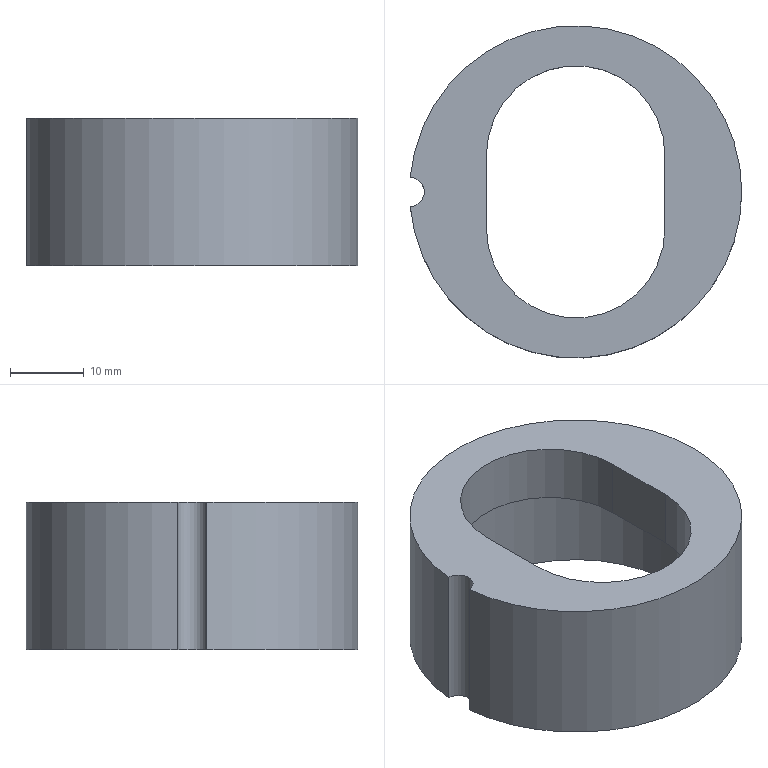Part | NX | features solid 2 | 1 solid | 10 faces | box 44.911 x 45 x 20 mm | volume 13855 mm3 | cylinder 5 | plane 5 | commonest cylinder face diameters 24.2 x2 4 x1 36 x1 45 x1
STEP:
#1=CARTESIAN_POINT('',(32.413,-54.637,-113.));
#2=VERTEX_POINT('',#1);
#3=CARTESIAN_POINT('',(32.413,-54.637,-93.));
#4=VERTEX_POINT('',#3);
#5=CARTESIAN_POINT('',(32.413,-54.637,-103.));
#6=DIRECTION('',(0.,0.,1.));
#7=VECTOR('',#6,1000.);
#8=LINE('',#5,#7);
#9=EDGE_CURVE('',#2,#4,#8,.T.);
#10=ORIENTED_EDGE('',*,*,#9,.F.);
#11=CARTESIAN_POINT('',(32.413,-50.641,-113.));
#12=VERTEX_POINT('',#11);
#13=CARTESIAN_POINT('',(54.824,-52.639,-113.));
#14=DIRECTION('',(0.,0.,1.));
#15=DIRECTION('',(-1.,0.,0.));
#16=AXIS2_PLACEMENT_3D('',#13,#14,#15);
#17=CIRCLE('',#16,22.5);
#18=EDGE_CURVE('',#2,#12,#17,.T.);
#19=ORIENTED_EDGE('',*,*,#18,.T.);
#20=CARTESIAN_POINT('',(32.413,-50.641,-93.));
#21=VERTEX_POINT('',#20);
#22=CARTESIAN_POINT('',(32.413,-50.641,-103.));
#23=DIRECTION('',(0.,0.,1.));
#24=VECTOR('',#23,1000.);
#25=LINE('',#22,#24);
#26=EDGE_CURVE('',#21,#12,#25,.F.);
#27=ORIENTED_EDGE('',*,*,#26,.F.);
#28=CARTESIAN_POINT('',(54.824,-52.639,-93.));
#29=DIRECTION('',(0.,0.,1.));
#30=DIRECTION('',(-1.,0.,0.));
#31=AXIS2_PLACEMENT_3D('',#28,#29,#30);
#32=CIRCLE('',#31,22.5);
#33=EDGE_CURVE('',#4,#21,#32,.T.);
#34=ORIENTED_EDGE('',*,*,#33,.F.);
#35=EDGE_LOOP('',(#10,#19,#27,#34));
#36=FACE_BOUND('',#35,.T.);
#37=CARTESIAN_POINT('',(54.824,-52.639,-113.));
#38=DIRECTION('',(0.,0.,1.));
#39=DIRECTION('',(-1.,0.,0.));
#40=AXIS2_PLACEMENT_3D('',#37,#38,#39);
#41=CYLINDRICAL_SURFACE('',#40,22.5);
#42=ADVANCED_FACE('',(#36),#41,.T.);
#43=CARTESIAN_POINT('',(36.824,-52.639,-113.));
#44=VERTEX_POINT('',#43);
#45=CARTESIAN_POINT('',(54.824,-52.639,-113.));
#46=DIRECTION('',(0.,0.,1.));
#47=DIRECTION('',(-1.,0.,0.));
#48=AXIS2_PLACEMENT_3D('',#45,#46,#47);
#49=CIRCLE('',#48,18.);
#50=EDGE_CURVE('',#44,#44,#49,.T.);
#51=ORIENTED_EDGE('',*,*,#50,.T.);
#52=EDGE_LOOP('',(#51));
#53=FACE_BOUND('',#52,.T.);
#54=ORIENTED_EDGE('',*,*,#18,.F.);
#55=CARTESIAN_POINT('',(32.324,-52.639,-113.));
#56=DIRECTION('',(0.,0.,1.));
#57=DIRECTION('',(-1.,0.,0.));
#58=AXIS2_PLACEMENT_3D('',#55,#56,#57);
#59=CIRCLE('',#58,2.);
#60=EDGE_CURVE('',#2,#12,#59,.T.);
#61=ORIENTED_EDGE('',*,*,#60,.T.);
#62=EDGE_LOOP('',(#54,#61));
#63=FACE_BOUND('',#62,.T.);
#64=CARTESIAN_POINT('',(54.824,-52.639,-113.));
#65=DIRECTION('',(0.,0.,1.));
#66=DIRECTION('',(-1.,0.,0.));
#67=AXIS2_PLACEMENT_3D('',#64,#65,#66);
#68=PLANE('',#67);
#69=ADVANCED_FACE('',(#53,#63),#68,.F.);
#70=CARTESIAN_POINT('',(66.924,-57.639,-93.));
#71=VERTEX_POINT('',#70);
#72=CARTESIAN_POINT('',(66.924,-47.639,-93.));
#73=VERTEX_POINT('',#72);
#74=CARTESIAN_POINT('',(66.924,-57.639,-93.));
#75=DIRECTION('',(0.,1.,0.));
#76=VECTOR('',#75,1000.);
#77=LINE('',#74,#76);
#78=EDGE_CURVE('',#71,#73,#77,.T.);
#79=ORIENTED_EDGE('',*,*,#78,.F.);
#80=CARTESIAN_POINT('',(42.724,-57.639,-93.));
#81=VERTEX_POINT('',#80);
#82=CARTESIAN_POINT('',(54.824,-57.639,-93.));
#83=DIRECTION('',(0.,0.,1.));
#84=DIRECTION('',(-1.,0.,0.));
#85=AXIS2_PLACEMENT_3D('',#82,#83,#84);
#86=CIRCLE('',#85,12.1);
#87=EDGE_CURVE('',#81,#71,#86,.T.);
#88=ORIENTED_EDGE('',*,*,#87,.F.);
#89=CARTESIAN_POINT('',(42.724,-47.639,-93.));
#90=VERTEX_POINT('',#89);
#91=CARTESIAN_POINT('',(42.724,-57.639,-93.));
#92=DIRECTION('',(0.,1.,0.));
#93=VECTOR('',#92,1000.);
#94=LINE('',#91,#93);
#95=EDGE_CURVE('',#81,#90,#94,.T.);
#96=ORIENTED_EDGE('',*,*,#95,.T.);
#97=CARTESIAN_POINT('',(54.824,-47.639,-93.));
#98=DIRECTION('',(0.,0.,1.));
#99=DIRECTION('',(-1.,0.,0.));
#100=AXIS2_PLACEMENT_3D('',#97,#98,#99);
#101=CIRCLE('',#100,12.1);
#102=EDGE_CURVE('',#73,#90,#101,.T.);
#103=ORIENTED_EDGE('',*,*,#102,.F.);
#104=EDGE_LOOP('',(#79,#88,#96,#103));
#105=FACE_BOUND('',#104,.T.);
#106=CARTESIAN_POINT('',(32.324,-52.639,-93.));
#107=DIRECTION('',(0.,0.,1.));
#108=DIRECTION('',(-1.,0.,0.));
#109=AXIS2_PLACEMENT_3D('',#106,#107,#108);
#110=CIRCLE('',#109,2.);
#111=EDGE_CURVE('',#4,#21,#110,.T.);
#112=ORIENTED_EDGE('',*,*,#111,.F.);
#113=ORIENTED_EDGE('',*,*,#33,.T.);
#114=EDGE_LOOP('',(#112,#113));
#115=FACE_BOUND('',#114,.T.);
#116=CARTESIAN_POINT('',(54.824,-52.639,-93.));
#117=DIRECTION('',(0.,0.,1.));
#118=DIRECTION('',(-1.,0.,0.));
#119=AXIS2_PLACEMENT_3D('',#116,#117,#118);
#120=PLANE('',#119);
#121=ADVANCED_FACE('',(#105,#115),#120,.T.);
#122=ORIENTED_EDGE('',*,*,#50,.F.);
#123=EDGE_LOOP('',(#122));
#124=FACE_BOUND('',#123,.T.);
#125=CARTESIAN_POINT('',(36.824,-52.639,-101.));
#126=VERTEX_POINT('',#125);
#127=CARTESIAN_POINT('',(54.824,-52.639,-101.));
#128=DIRECTION('',(0.,0.,1.));
#129=DIRECTION('',(-1.,0.,0.));
#130=AXIS2_PLACEMENT_3D('',#127,#128,#129);
#131=CIRCLE('',#130,18.);
#132=EDGE_CURVE('',#126,#126,#131,.T.);
#133=ORIENTED_EDGE('',*,*,#132,.T.);
#134=EDGE_LOOP('',(#133));
#135=FACE_BOUND('',#134,.T.);
#136=CARTESIAN_POINT('',(54.824,-52.639,-113.));
#137=DIRECTION('',(0.,0.,1.));
#138=DIRECTION('',(-1.,0.,0.));
#139=AXIS2_PLACEMENT_3D('',#136,#137,#138);
#140=CYLINDRICAL_SURFACE('',#139,18.);
#141=ADVANCED_FACE('',(#124,#135),#140,.F.);
#142=CARTESIAN_POINT('',(42.724,-57.639,-101.));
#143=VERTEX_POINT('',#142);
#144=CARTESIAN_POINT('',(66.924,-57.639,-101.));
#145=VERTEX_POINT('',#144);
#146=CARTESIAN_POINT('',(54.824,-57.639,-101.));
#147=DIRECTION('',(0.,0.,1.));
#148=DIRECTION('',(-1.,0.,0.));
#149=AXIS2_PLACEMENT_3D('',#146,#147,#148);
#150=CIRCLE('',#149,12.1);
#151=EDGE_CURVE('',#143,#145,#150,.T.);
#152=ORIENTED_EDGE('',*,*,#151,.T.);
#153=CARTESIAN_POINT('',(66.924,-47.639,-101.));
#154=VERTEX_POINT('',#153);
#155=CARTESIAN_POINT('',(66.924,-52.639,-101.));
#156=DIRECTION('',(0.,1.,0.));
#157=VECTOR('',#156,1000.);
#158=LINE('',#155,#157);
#159=EDGE_CURVE('',#145,#154,#158,.T.);
#160=ORIENTED_EDGE('',*,*,#159,.T.);
#161=CARTESIAN_POINT('',(42.724,-47.639,-101.));
#162=VERTEX_POINT('',#161);
#163=CARTESIAN_POINT('',(54.824,-47.639,-101.));
#164=DIRECTION('',(0.,0.,1.));
#165=DIRECTION('',(-1.,0.,0.));
#166=AXIS2_PLACEMENT_3D('',#163,#164,#165);
#167=CIRCLE('',#166,12.1);
#168=EDGE_CURVE('',#154,#162,#167,.T.);
#169=ORIENTED_EDGE('',*,*,#168,.T.);
#170=CARTESIAN_POINT('',(42.724,-52.639,-101.));
#171=DIRECTION('',(0.,1.,0.));
#172=VECTOR('',#171,1000.);
#173=LINE('',#170,#172);
#174=EDGE_CURVE('',#143,#162,#173,.T.);
#175=ORIENTED_EDGE('',*,*,#174,.F.);
#176=EDGE_LOOP('',(#152,#160,#169,#175));
#177=FACE_BOUND('',#176,.T.);
#178=ORIENTED_EDGE('',*,*,#132,.F.);
#179=EDGE_LOOP('',(#178));
#180=FACE_BOUND('',#179,.T.);
#181=CARTESIAN_POINT('',(54.824,-52.639,-101.));
#182=DIRECTION('',(0.,0.,1.));
#183=DIRECTION('',(-1.,0.,0.));
#184=AXIS2_PLACEMENT_3D('',#181,#182,#183);
#185=PLANE('',#184);
#186=ADVANCED_FACE('',(#177,#180),#185,.F.);
#187=ORIENTED_EDGE('',*,*,#9,.T.);
#188=ORIENTED_EDGE('',*,*,#111,.T.);
#189=ORIENTED_EDGE('',*,*,#26,.T.);
#190=ORIENTED_EDGE('',*,*,#60,.F.);
#191=EDGE_LOOP('',(#187,#188,#189,#190));
#192=FACE_BOUND('',#191,.T.);
#193=CARTESIAN_POINT('',(32.324,-52.639,-113.));
#194=DIRECTION('',(0.,0.,1.));
#195=DIRECTION('',(-1.,0.,0.));
#196=AXIS2_PLACEMENT_3D('',#193,#194,#195);
#197=CYLINDRICAL_SURFACE('',#196,2.);
#198=ADVANCED_FACE('',(#192),#197,.F.);
#199=CARTESIAN_POINT('',(66.924,-57.639,-113.));
#200=DIRECTION('',(0.,0.,1.));
#201=VECTOR('',#200,1000.);
#202=LINE('',#199,#201);
#203=EDGE_CURVE('',#145,#71,#202,.T.);
#204=ORIENTED_EDGE('',*,*,#203,.T.);
#205=ORIENTED_EDGE('',*,*,#78,.T.);
#206=CARTESIAN_POINT('',(66.924,-47.639,-113.));
#207=DIRECTION('',(0.,0.,1.));
#208=VECTOR('',#207,1000.);
#209=LINE('',#206,#208);
#210=EDGE_CURVE('',#154,#73,#209,.T.);
#211=ORIENTED_EDGE('',*,*,#210,.F.);
#212=ORIENTED_EDGE('',*,*,#159,.F.);
#213=EDGE_LOOP('',(#204,#205,#211,#212));
#214=FACE_BOUND('',#213,.T.);
#215=CARTESIAN_POINT('',(66.924,-57.639,-113.));
#216=DIRECTION('',(1.,0.,0.));
#217=DIRECTION('',(0.,0.,1.));
#218=AXIS2_PLACEMENT_3D('',#215,#216,#217);
#219=PLANE('',#218);
#220=ADVANCED_FACE('',(#214),#219,.F.);
#221=ORIENTED_EDGE('',*,*,#210,.T.);
#222=ORIENTED_EDGE('',*,*,#102,.T.);
#223=CARTESIAN_POINT('',(42.724,-47.639,-113.));
#224=DIRECTION('',(0.,0.,1.));
#225=VECTOR('',#224,1000.);
#226=LINE('',#223,#225);
#227=EDGE_CURVE('',#162,#90,#226,.T.);
#228=ORIENTED_EDGE('',*,*,#227,.F.);
#229=ORIENTED_EDGE('',*,*,#168,.F.);
#230=EDGE_LOOP('',(#221,#222,#228,#229));
#231=FACE_BOUND('',#230,.T.);
#232=CARTESIAN_POINT('',(54.824,-47.639,-113.));
#233=DIRECTION('',(0.,0.,1.));
#234=DIRECTION('',(-1.,0.,0.));
#235=AXIS2_PLACEMENT_3D('',#232,#233,#234);
#236=CYLINDRICAL_SURFACE('',#235,12.1);
#237=ADVANCED_FACE('',(#231),#236,.F.);
#238=ORIENTED_EDGE('',*,*,#174,.T.);
#239=ORIENTED_EDGE('',*,*,#227,.T.);
#240=ORIENTED_EDGE('',*,*,#95,.F.);
#241=CARTESIAN_POINT('',(42.724,-57.639,-113.));
#242=DIRECTION('',(0.,0.,1.));
#243=VECTOR('',#242,1000.);
#244=LINE('',#241,#243);
#245=EDGE_CURVE('',#143,#81,#244,.T.);
#246=ORIENTED_EDGE('',*,*,#245,.F.);
#247=EDGE_LOOP('',(#238,#239,#240,#246));
#248=FACE_BOUND('',#247,.T.);
#249=CARTESIAN_POINT('',(42.724,-57.639,-113.));
#250=DIRECTION('',(1.,0.,0.));
#251=DIRECTION('',(0.,0.,1.));
#252=AXIS2_PLACEMENT_3D('',#249,#250,#251);
#253=PLANE('',#252);
#254=ADVANCED_FACE('',(#248),#253,.T.);
#255=ORIENTED_EDGE('',*,*,#245,.T.);
#256=ORIENTED_EDGE('',*,*,#87,.T.);
#257=ORIENTED_EDGE('',*,*,#203,.F.);
#258=ORIENTED_EDGE('',*,*,#151,.F.);
#259=EDGE_LOOP('',(#255,#256,#257,#258));
#260=FACE_BOUND('',#259,.T.);
#261=CARTESIAN_POINT('',(54.824,-57.639,-113.));
#262=DIRECTION('',(0.,0.,1.));
#263=DIRECTION('',(-1.,0.,0.));
#264=AXIS2_PLACEMENT_3D('',#261,#262,#263);
#265=CYLINDRICAL_SURFACE('',#264,12.1);
#266=ADVANCED_FACE('',(#260),#265,.F.);
#267=CLOSED_SHELL('',(#42,#69,#121,#141,#186,#198,#220,#237,#254,#266));
#268=MANIFOLD_SOLID_BREP('',#267);
#269=(LENGTH_UNIT()NAMED_UNIT(*)SI_UNIT(.MILLI.,.METRE.));
#270=UNCERTAINTY_MEASURE_WITH_UNIT(LENGTH_MEASURE(0.00001),#269,'','');
#271=(NAMED_UNIT(*)PLANE_ANGLE_UNIT()SI_UNIT($,.RADIAN.));
#272=(NAMED_UNIT(*)SI_UNIT($,.STERADIAN.)SOLID_ANGLE_UNIT());
#273=(GEOMETRIC_REPRESENTATION_CONTEXT(3)GLOBAL_UNCERTAINTY_ASSIGNED_CONTEXT((#270))GLOBAL_UNIT_ASSIGNED_CONTEXT((#269,#271,#272))REPRESENTATION_CONTEXT('',''));
#274=ADVANCED_BREP_SHAPE_REPRESENTATION('',(#268),#273);